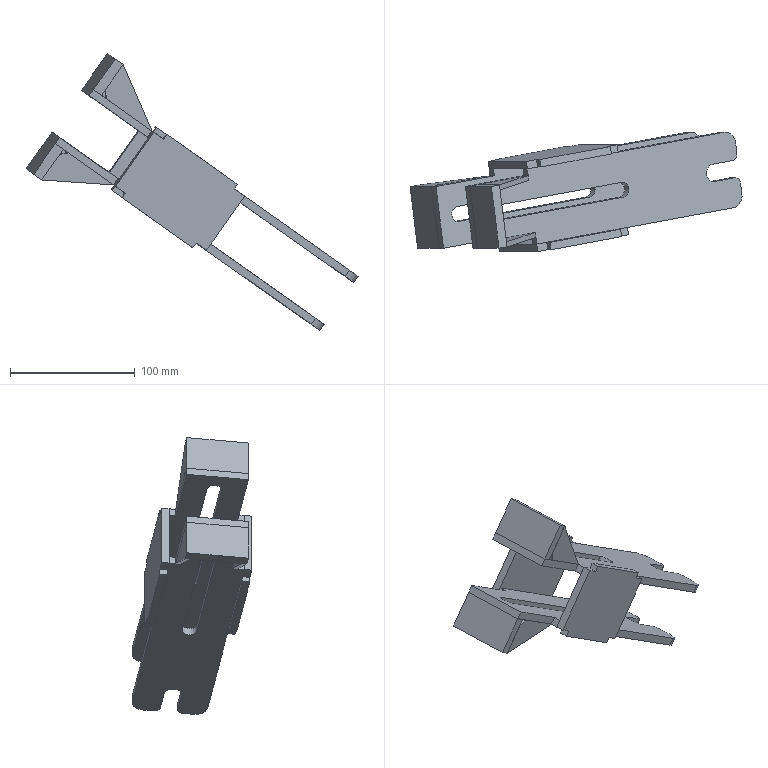Part | STEP file | HL4GZ-1.862.045 (tensioner wheel mounting frame) | 10 solids | 108 faces | box 265.962 x 95.725 x 221.775 mm | volume 259615 mm3 | plane 94 | cylinder 14 | commonest cylinder face diameters 10 x4 12 x4 20 x4 14 x2